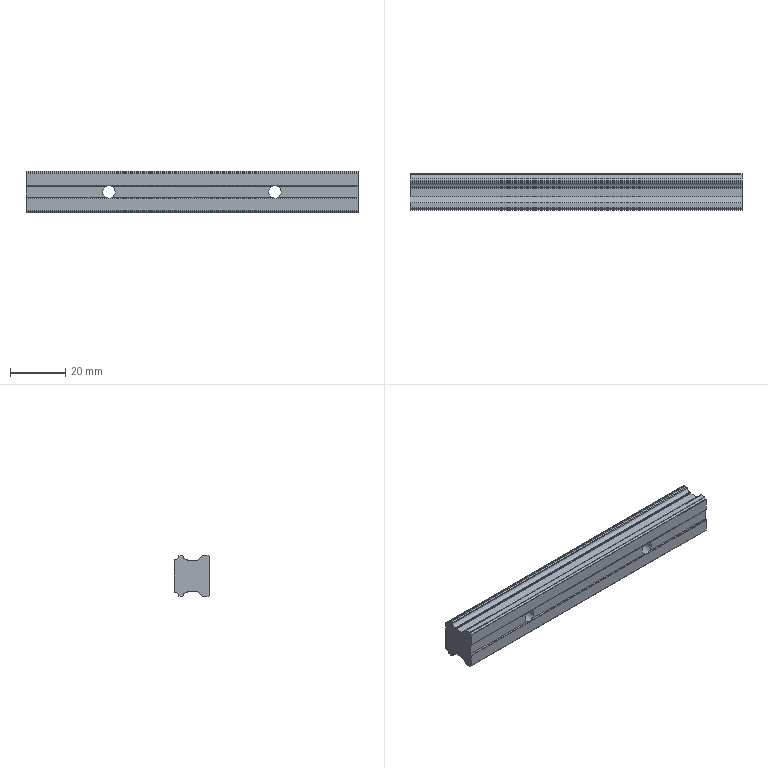Part | STEP file | SHS15C12030_Track | 1 solid | 60 faces | box 120 x 13 x 15 mm | volume 19221 mm3 | plane 30 | cylinder 30 | commonest cylinder face diameters 0.6 x6 2.861 x4 0.398 x2 0.545 x2 0.558 x2 0.626 x2